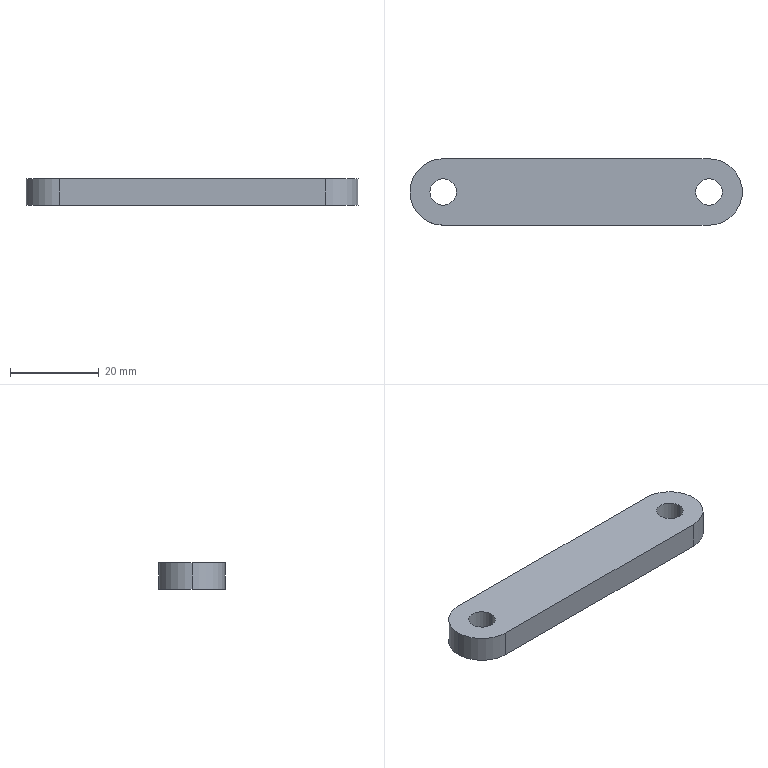Part | SolidWorks | features Extrusion 1 | 1 solid | 11 faces | box 75 x 15 x 6 mm | volume 6121 mm3 | cylinder 7 | plane 4 | commonest cylinder face diameters 6 x4 15 x3
STEP:
#1=CARTESIAN_POINT('',(57.,0.,6.));
#2=VERTEX_POINT('',#1);
#3=CARTESIAN_POINT('',(63.,0.,6.));
#4=VERTEX_POINT('',#3);
#5=CARTESIAN_POINT('',(60.,0.,6.));
#6=DIRECTION('',(0.,0.,1.));
#7=DIRECTION('',(1.,0.,0.));
#8=AXIS2_PLACEMENT_3D('',#5,#6,#7);
#9=CIRCLE('',#8,3.);
#10=EDGE_CURVE('',#2,#4,#9,.T.);
#11=ORIENTED_EDGE('',*,*,#10,.T.);
#12=CARTESIAN_POINT('',(63.,0.,0.));
#13=VERTEX_POINT('',#12);
#14=CARTESIAN_POINT('',(63.,0.,6.));
#15=DIRECTION('',(0.,0.,-1.));
#16=VECTOR('',#15,1000.);
#17=LINE('',#14,#16);
#18=EDGE_CURVE('',#4,#13,#17,.T.);
#19=ORIENTED_EDGE('',*,*,#18,.T.);
#20=CARTESIAN_POINT('',(57.,0.,0.));
#21=VERTEX_POINT('',#20);
#22=CARTESIAN_POINT('',(60.,0.,0.));
#23=DIRECTION('',(0.,0.,1.));
#24=DIRECTION('',(1.,0.,0.));
#25=AXIS2_PLACEMENT_3D('',#22,#23,#24);
#26=CIRCLE('',#25,3.);
#27=EDGE_CURVE('',#21,#13,#26,.T.);
#28=ORIENTED_EDGE('',*,*,#27,.F.);
#29=CARTESIAN_POINT('',(57.,0.,6.));
#30=DIRECTION('',(0.,0.,-1.));
#31=VECTOR('',#30,1000.);
#32=LINE('',#29,#31);
#33=EDGE_CURVE('',#2,#21,#32,.T.);
#34=ORIENTED_EDGE('',*,*,#33,.F.);
#35=EDGE_LOOP('',(#11,#19,#28,#34));
#36=FACE_OUTER_BOUND('',#35,.T.);
#37=CARTESIAN_POINT('',(60.,0.,6.));
#38=DIRECTION('',(0.,0.,-1.));
#39=DIRECTION('',(-1.,0.,0.));
#40=AXIS2_PLACEMENT_3D('',#37,#38,#39);
#41=CYLINDRICAL_SURFACE('',#40,3.);
#42=ADVANCED_FACE('',(#36),#41,.F.);
#43=CARTESIAN_POINT('',(-3.,0.,6.));
#44=VERTEX_POINT('',#43);
#45=CARTESIAN_POINT('',(3.,0.,6.));
#46=VERTEX_POINT('',#45);
#47=CARTESIAN_POINT('',(0.,0.,6.));
#48=DIRECTION('',(0.,0.,1.));
#49=DIRECTION('',(1.,0.,0.));
#50=AXIS2_PLACEMENT_3D('',#47,#48,#49);
#51=CIRCLE('',#50,3.);
#52=EDGE_CURVE('',#44,#46,#51,.T.);
#53=ORIENTED_EDGE('',*,*,#52,.T.);
#54=CARTESIAN_POINT('',(3.,0.,0.));
#55=VERTEX_POINT('',#54);
#56=CARTESIAN_POINT('',(3.,0.,6.));
#57=DIRECTION('',(0.,0.,-1.));
#58=VECTOR('',#57,1000.);
#59=LINE('',#56,#58);
#60=EDGE_CURVE('',#46,#55,#59,.T.);
#61=ORIENTED_EDGE('',*,*,#60,.T.);
#62=CARTESIAN_POINT('',(-3.,0.,0.));
#63=VERTEX_POINT('',#62);
#64=CARTESIAN_POINT('',(0.,0.,0.));
#65=DIRECTION('',(0.,0.,1.));
#66=DIRECTION('',(1.,0.,0.));
#67=AXIS2_PLACEMENT_3D('',#64,#65,#66);
#68=CIRCLE('',#67,3.);
#69=EDGE_CURVE('',#63,#55,#68,.T.);
#70=ORIENTED_EDGE('',*,*,#69,.F.);
#71=CARTESIAN_POINT('',(-3.,0.,6.));
#72=DIRECTION('',(0.,0.,-1.));
#73=VECTOR('',#72,1000.);
#74=LINE('',#71,#73);
#75=EDGE_CURVE('',#44,#63,#74,.T.);
#76=ORIENTED_EDGE('',*,*,#75,.F.);
#77=EDGE_LOOP('',(#53,#61,#70,#76));
#78=FACE_OUTER_BOUND('',#77,.T.);
#79=CARTESIAN_POINT('',(0.,0.,6.));
#80=DIRECTION('',(0.,0.,-1.));
#81=DIRECTION('',(-1.,0.,0.));
#82=AXIS2_PLACEMENT_3D('',#79,#80,#81);
#83=CYLINDRICAL_SURFACE('',#82,3.);
#84=ADVANCED_FACE('',(#78),#83,.F.);
#85=CARTESIAN_POINT('',(-7.5,0.,6.));
#86=VERTEX_POINT('',#85);
#87=CARTESIAN_POINT('',(0.,-7.5,6.));
#88=VERTEX_POINT('',#87);
#89=CARTESIAN_POINT('',(0.,0.,6.));
#90=DIRECTION('',(0.,0.,1.));
#91=DIRECTION('',(1.,0.,0.));
#92=AXIS2_PLACEMENT_3D('',#89,#90,#91);
#93=CIRCLE('',#92,7.5);
#94=EDGE_CURVE('',#86,#88,#93,.T.);
#95=ORIENTED_EDGE('',*,*,#94,.F.);
#96=CARTESIAN_POINT('',(-7.5,0.,0.));
#97=VERTEX_POINT('',#96);
#98=CARTESIAN_POINT('',(-7.5,0.,6.));
#99=DIRECTION('',(0.,0.,-1.));
#100=VECTOR('',#99,1000.);
#101=LINE('',#98,#100);
#102=EDGE_CURVE('',#86,#97,#101,.T.);
#103=ORIENTED_EDGE('',*,*,#102,.T.);
#104=CARTESIAN_POINT('',(0.,-7.5,0.));
#105=VERTEX_POINT('',#104);
#106=CARTESIAN_POINT('',(0.,0.,0.));
#107=DIRECTION('',(0.,0.,1.));
#108=DIRECTION('',(1.,0.,0.));
#109=AXIS2_PLACEMENT_3D('',#106,#107,#108);
#110=CIRCLE('',#109,7.5);
#111=EDGE_CURVE('',#97,#105,#110,.T.);
#112=ORIENTED_EDGE('',*,*,#111,.T.);
#113=CARTESIAN_POINT('',(0.,-7.5,6.));
#114=DIRECTION('',(0.,0.,-1.));
#115=VECTOR('',#114,1000.);
#116=LINE('',#113,#115);
#117=EDGE_CURVE('',#88,#105,#116,.T.);
#118=ORIENTED_EDGE('',*,*,#117,.F.);
#119=EDGE_LOOP('',(#95,#103,#112,#118));
#120=FACE_OUTER_BOUND('',#119,.T.);
#121=CARTESIAN_POINT('',(0.,0.,6.));
#122=DIRECTION('',(0.,0.,-1.));
#123=DIRECTION('',(-1.,0.,0.));
#124=AXIS2_PLACEMENT_3D('',#121,#122,#123);
#125=CYLINDRICAL_SURFACE('',#124,7.5);
#126=ADVANCED_FACE('',(#120),#125,.T.);
#127=ORIENTED_EDGE('',*,*,#52,.F.);
#128=CARTESIAN_POINT('',(0.,0.,6.));
#129=DIRECTION('',(0.,0.,1.));
#130=DIRECTION('',(1.,0.,0.));
#131=AXIS2_PLACEMENT_3D('',#128,#129,#130);
#132=CIRCLE('',#131,3.);
#133=EDGE_CURVE('',#46,#44,#132,.T.);
#134=ORIENTED_EDGE('',*,*,#133,.F.);
#135=EDGE_LOOP('',(#127,#134));
#136=FACE_BOUND('',#135,.T.);
#137=CARTESIAN_POINT('',(0.,7.5,6.));
#138=VERTEX_POINT('',#137);
#139=CARTESIAN_POINT('',(0.,0.,6.));
#140=DIRECTION('',(0.,0.,1.));
#141=DIRECTION('',(1.,0.,0.));
#142=AXIS2_PLACEMENT_3D('',#139,#140,#141);
#143=CIRCLE('',#142,7.5);
#144=EDGE_CURVE('',#138,#86,#143,.T.);
#145=ORIENTED_EDGE('',*,*,#144,.T.);
#146=ORIENTED_EDGE('',*,*,#94,.T.);
#147=CARTESIAN_POINT('',(60.,-7.5,6.));
#148=VERTEX_POINT('',#147);
#149=CARTESIAN_POINT('',(0.,-7.5,6.));
#150=DIRECTION('',(1.,0.,0.));
#151=VECTOR('',#150,1000.);
#152=LINE('',#149,#151);
#153=EDGE_CURVE('',#88,#148,#152,.T.);
#154=ORIENTED_EDGE('',*,*,#153,.T.);
#155=CARTESIAN_POINT('',(60.,7.5,6.));
#156=VERTEX_POINT('',#155);
#157=CARTESIAN_POINT('',(60.,0.,6.));
#158=DIRECTION('',(0.,0.,1.));
#159=DIRECTION('',(1.,0.,0.));
#160=AXIS2_PLACEMENT_3D('',#157,#158,#159);
#161=CIRCLE('',#160,7.5);
#162=EDGE_CURVE('',#148,#156,#161,.T.);
#163=ORIENTED_EDGE('',*,*,#162,.T.);
#164=CARTESIAN_POINT('',(0.,7.5,6.));
#165=DIRECTION('',(-1.,0.,0.));
#166=VECTOR('',#165,1000.);
#167=LINE('',#164,#166);
#168=EDGE_CURVE('',#156,#138,#167,.T.);
#169=ORIENTED_EDGE('',*,*,#168,.T.);
#170=EDGE_LOOP('',(#145,#146,#154,#163,#169));
#171=FACE_OUTER_BOUND('',#170,.T.);
#172=ORIENTED_EDGE('',*,*,#10,.F.);
#173=CARTESIAN_POINT('',(60.,0.,6.));
#174=DIRECTION('',(0.,0.,1.));
#175=DIRECTION('',(1.,0.,0.));
#176=AXIS2_PLACEMENT_3D('',#173,#174,#175);
#177=CIRCLE('',#176,3.);
#178=EDGE_CURVE('',#4,#2,#177,.T.);
#179=ORIENTED_EDGE('',*,*,#178,.F.);
#180=EDGE_LOOP('',(#172,#179));
#181=FACE_BOUND('',#180,.T.);
#182=CARTESIAN_POINT('',(0.,0.,6.));
#183=DIRECTION('',(0.,0.,1.));
#184=DIRECTION('',(1.,0.,0.));
#185=AXIS2_PLACEMENT_3D('',#182,#183,#184);
#186=PLANE('',#185);
#187=ADVANCED_FACE('',(#136,#171,#181),#186,.T.);
#188=CARTESIAN_POINT('',(0.,7.5,0.));
#189=VERTEX_POINT('',#188);
#190=CARTESIAN_POINT('',(0.,0.,0.));
#191=DIRECTION('',(0.,0.,1.));
#192=DIRECTION('',(1.,0.,0.));
#193=AXIS2_PLACEMENT_3D('',#190,#191,#192);
#194=CIRCLE('',#193,7.5);
#195=EDGE_CURVE('',#189,#97,#194,.T.);
#196=ORIENTED_EDGE('',*,*,#195,.F.);
#197=CARTESIAN_POINT('',(60.,7.5,0.));
#198=VERTEX_POINT('',#197);
#199=CARTESIAN_POINT('',(0.,7.5,0.));
#200=DIRECTION('',(-1.,0.,0.));
#201=VECTOR('',#200,1000.);
#202=LINE('',#199,#201);
#203=EDGE_CURVE('',#198,#189,#202,.T.);
#204=ORIENTED_EDGE('',*,*,#203,.F.);
#205=CARTESIAN_POINT('',(60.,-7.5,0.));
#206=VERTEX_POINT('',#205);
#207=CARTESIAN_POINT('',(60.,0.,0.));
#208=DIRECTION('',(0.,0.,1.));
#209=DIRECTION('',(1.,0.,0.));
#210=AXIS2_PLACEMENT_3D('',#207,#208,#209);
#211=CIRCLE('',#210,7.5);
#212=EDGE_CURVE('',#206,#198,#211,.T.);
#213=ORIENTED_EDGE('',*,*,#212,.F.);
#214=CARTESIAN_POINT('',(0.,-7.5,0.));
#215=DIRECTION('',(1.,0.,0.));
#216=VECTOR('',#215,1000.);
#217=LINE('',#214,#216);
#218=EDGE_CURVE('',#105,#206,#217,.T.);
#219=ORIENTED_EDGE('',*,*,#218,.F.);
#220=ORIENTED_EDGE('',*,*,#111,.F.);
#221=EDGE_LOOP('',(#196,#204,#213,#219,#220));
#222=FACE_OUTER_BOUND('',#221,.T.);
#223=ORIENTED_EDGE('',*,*,#69,.T.);
#224=CARTESIAN_POINT('',(0.,0.,0.));
#225=DIRECTION('',(0.,0.,1.));
#226=DIRECTION('',(1.,0.,0.));
#227=AXIS2_PLACEMENT_3D('',#224,#225,#226);
#228=CIRCLE('',#227,3.);
#229=EDGE_CURVE('',#55,#63,#228,.T.);
#230=ORIENTED_EDGE('',*,*,#229,.T.);
#231=EDGE_LOOP('',(#223,#230));
#232=FACE_BOUND('',#231,.T.);
#233=ORIENTED_EDGE('',*,*,#27,.T.);
#234=CARTESIAN_POINT('',(60.,0.,0.));
#235=DIRECTION('',(0.,0.,1.));
#236=DIRECTION('',(1.,0.,0.));
#237=AXIS2_PLACEMENT_3D('',#234,#235,#236);
#238=CIRCLE('',#237,3.);
#239=EDGE_CURVE('',#13,#21,#238,.T.);
#240=ORIENTED_EDGE('',*,*,#239,.T.);
#241=EDGE_LOOP('',(#233,#240));
#242=FACE_BOUND('',#241,.T.);
#243=CARTESIAN_POINT('',(0.,0.,0.));
#244=DIRECTION('',(0.,0.,1.));
#245=DIRECTION('',(1.,0.,0.));
#246=AXIS2_PLACEMENT_3D('',#243,#244,#245);
#247=PLANE('',#246);
#248=ADVANCED_FACE('',(#222,#232,#242),#247,.F.);
#249=ORIENTED_EDGE('',*,*,#102,.F.);
#250=ORIENTED_EDGE('',*,*,#144,.F.);
#251=CARTESIAN_POINT('',(0.,7.5,6.));
#252=DIRECTION('',(0.,0.,-1.));
#253=VECTOR('',#252,1000.);
#254=LINE('',#251,#253);
#255=EDGE_CURVE('',#138,#189,#254,.T.);
#256=ORIENTED_EDGE('',*,*,#255,.T.);
#257=ORIENTED_EDGE('',*,*,#195,.T.);
#258=EDGE_LOOP('',(#249,#250,#256,#257));
#259=FACE_OUTER_BOUND('',#258,.T.);
#260=CARTESIAN_POINT('',(0.,0.,6.));
#261=DIRECTION('',(0.,0.,-1.));
#262=DIRECTION('',(-1.,0.,0.));
#263=AXIS2_PLACEMENT_3D('',#260,#261,#262);
#264=CYLINDRICAL_SURFACE('',#263,7.5);
#265=ADVANCED_FACE('',(#259),#264,.T.);
#266=ORIENTED_EDGE('',*,*,#218,.T.);
#267=CARTESIAN_POINT('',(60.,-7.5,6.));
#268=DIRECTION('',(0.,0.,-1.));
#269=VECTOR('',#268,1000.);
#270=LINE('',#267,#269);
#271=EDGE_CURVE('',#148,#206,#270,.T.);
#272=ORIENTED_EDGE('',*,*,#271,.F.);
#273=ORIENTED_EDGE('',*,*,#153,.F.);
#274=ORIENTED_EDGE('',*,*,#117,.T.);
#275=EDGE_LOOP('',(#266,#272,#273,#274));
#276=FACE_OUTER_BOUND('',#275,.T.);
#277=CARTESIAN_POINT('',(0.,-7.5,6.));
#278=DIRECTION('',(0.,1.,0.));
#279=DIRECTION('',(-1.,0.,0.));
#280=AXIS2_PLACEMENT_3D('',#277,#278,#279);
#281=PLANE('',#280);
#282=ADVANCED_FACE('',(#276),#281,.F.);
#283=ORIENTED_EDGE('',*,*,#212,.T.);
#284=CARTESIAN_POINT('',(60.,7.5,6.));
#285=DIRECTION('',(0.,0.,-1.));
#286=VECTOR('',#285,1000.);
#287=LINE('',#284,#286);
#288=EDGE_CURVE('',#156,#198,#287,.T.);
#289=ORIENTED_EDGE('',*,*,#288,.F.);
#290=ORIENTED_EDGE('',*,*,#162,.F.);
#291=ORIENTED_EDGE('',*,*,#271,.T.);
#292=EDGE_LOOP('',(#283,#289,#290,#291));
#293=FACE_OUTER_BOUND('',#292,.T.);
#294=CARTESIAN_POINT('',(60.,0.,6.));
#295=DIRECTION('',(0.,0.,-1.));
#296=DIRECTION('',(-1.,0.,0.));
#297=AXIS2_PLACEMENT_3D('',#294,#295,#296);
#298=CYLINDRICAL_SURFACE('',#297,7.5);
#299=ADVANCED_FACE('',(#293),#298,.T.);
#300=ORIENTED_EDGE('',*,*,#203,.T.);
#301=ORIENTED_EDGE('',*,*,#255,.F.);
#302=ORIENTED_EDGE('',*,*,#168,.F.);
#303=ORIENTED_EDGE('',*,*,#288,.T.);
#304=EDGE_LOOP('',(#300,#301,#302,#303));
#305=FACE_OUTER_BOUND('',#304,.T.);
#306=CARTESIAN_POINT('',(0.,7.5,6.));
#307=DIRECTION('',(0.,-1.,0.));
#308=DIRECTION('',(1.,0.,0.));
#309=AXIS2_PLACEMENT_3D('',#306,#307,#308);
#310=PLANE('',#309);
#311=ADVANCED_FACE('',(#305),#310,.F.);
#312=ORIENTED_EDGE('',*,*,#60,.F.);
#313=ORIENTED_EDGE('',*,*,#133,.T.);
#314=ORIENTED_EDGE('',*,*,#75,.T.);
#315=ORIENTED_EDGE('',*,*,#229,.F.);
#316=EDGE_LOOP('',(#312,#313,#314,#315));
#317=FACE_OUTER_BOUND('',#316,.T.);
#318=CARTESIAN_POINT('',(0.,0.,6.));
#319=DIRECTION('',(0.,0.,-1.));
#320=DIRECTION('',(-1.,0.,0.));
#321=AXIS2_PLACEMENT_3D('',#318,#319,#320);
#322=CYLINDRICAL_SURFACE('',#321,3.);
#323=ADVANCED_FACE('',(#317),#322,.F.);
#324=ORIENTED_EDGE('',*,*,#18,.F.);
#325=ORIENTED_EDGE('',*,*,#178,.T.);
#326=ORIENTED_EDGE('',*,*,#33,.T.);
#327=ORIENTED_EDGE('',*,*,#239,.F.);
#328=EDGE_LOOP('',(#324,#325,#326,#327));
#329=FACE_OUTER_BOUND('',#328,.T.);
#330=CARTESIAN_POINT('',(60.,0.,6.));
#331=DIRECTION('',(0.,0.,-1.));
#332=DIRECTION('',(-1.,0.,0.));
#333=AXIS2_PLACEMENT_3D('',#330,#331,#332);
#334=CYLINDRICAL_SURFACE('',#333,3.);
#335=ADVANCED_FACE('',(#329),#334,.F.);
#336=CLOSED_SHELL('',(#42,#84,#126,#187,#248,#265,#282,#299,#311,#323,#335));
#337=MANIFOLD_SOLID_BREP('',#336);
#338=CARTESIAN_POINT('',(0.,0.,0.));
#339=DIRECTION('',(0.,0.,1.));
#340=DIRECTION('',(1.,0.,0.));
#341=AXIS2_PLACEMENT_3D('',#338,#339,#340);
#342=(LENGTH_UNIT()NAMED_UNIT(*)SI_UNIT(.MILLI.,.METRE.));
#343=UNCERTAINTY_MEASURE_WITH_UNIT(LENGTH_MEASURE(0.00001),#342,'','');
#344=(NAMED_UNIT(*)PLANE_ANGLE_UNIT()SI_UNIT($,.RADIAN.));
#345=(NAMED_UNIT(*)SI_UNIT($,.STERADIAN.)SOLID_ANGLE_UNIT());
#346=(GEOMETRIC_REPRESENTATION_CONTEXT(3)GLOBAL_UNCERTAINTY_ASSIGNED_CONTEXT((#343))GLOBAL_UNIT_ASSIGNED_CONTEXT((#342,#344,#345))REPRESENTATION_CONTEXT('',''));
#347=ADVANCED_BREP_SHAPE_REPRESENTATION('',(#337,#341),#346);